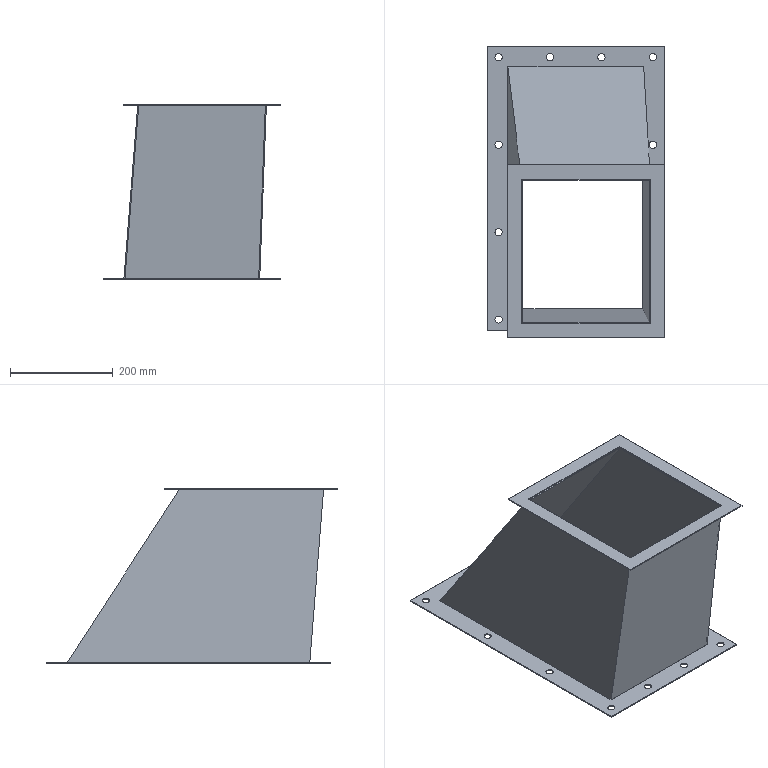Part | STEP file | Produce dryer line heating fan-OVEN-445 | 3 solids | 54 faces | box 345.008 x 567.391 x 339.5 mm | volume 1076631 mm3 | plane 30 | cylinder 24 | commonest cylinder face diameters 14 x24